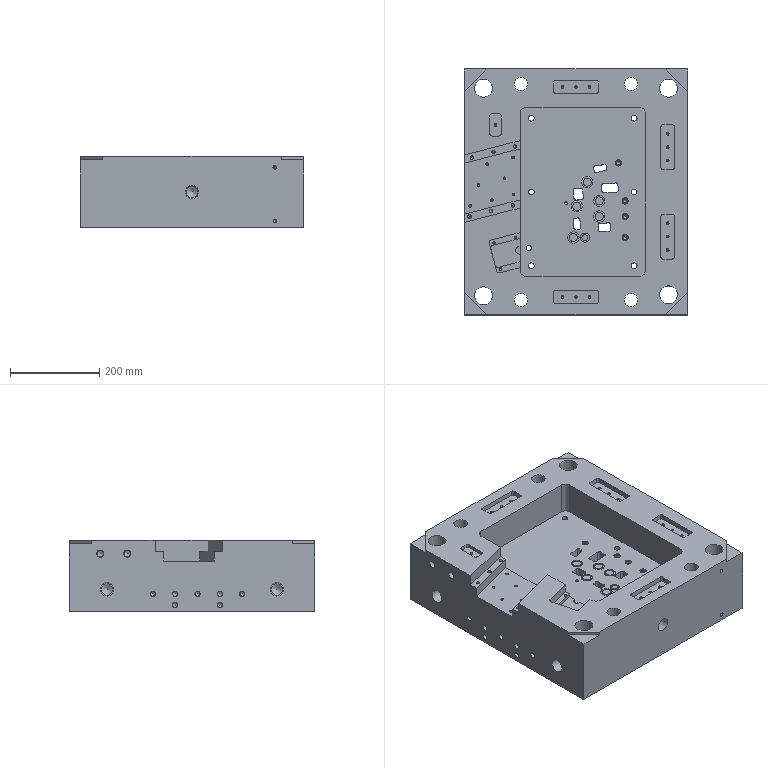Part | STEP file | 车灯-后视镜_id622_x_t | 1 solid | 540 faces | box 500 x 550 x 160 mm | volume 32899557 mm3 | cylinder 243 | plane 202 | cone 78 | spline 17 | commonest cylinder face diameters 8 x48 6 x24 6.9 x24 5.1 x23 10 x19 12 x12